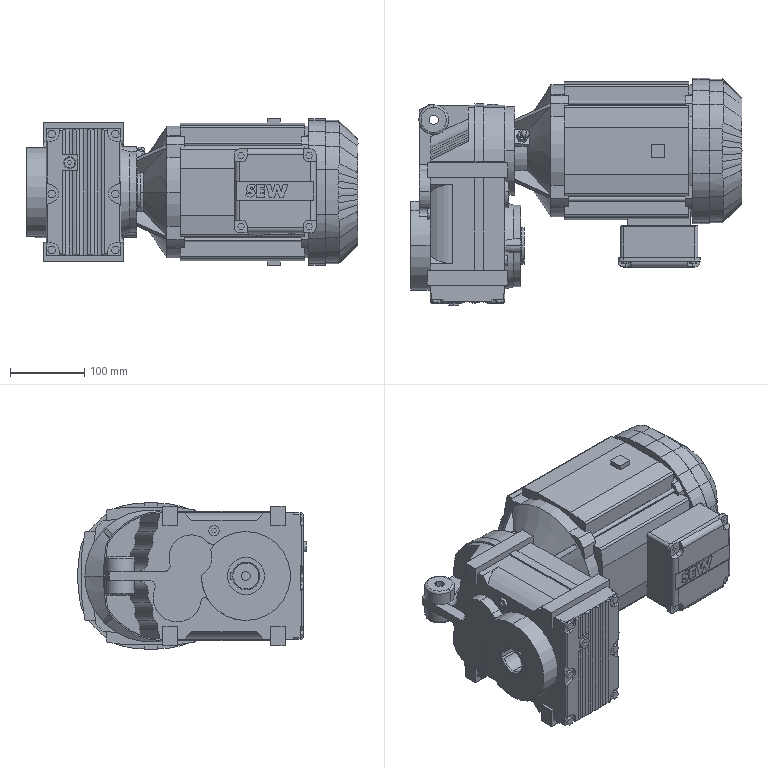Part | SolidWorks | features MBimport 1 | 2 solids | 806 faces | box 447.5 x 307.56 x 199 mm | volume 13556932 mm3 | plane 421 | cylinder 296 | cone 39 | spline 38 | torus 8 | sphere 4 | commonest cylinder face diameters 0.1 x29 14 x26 6 x20 24 x16 120 x13 20 x12